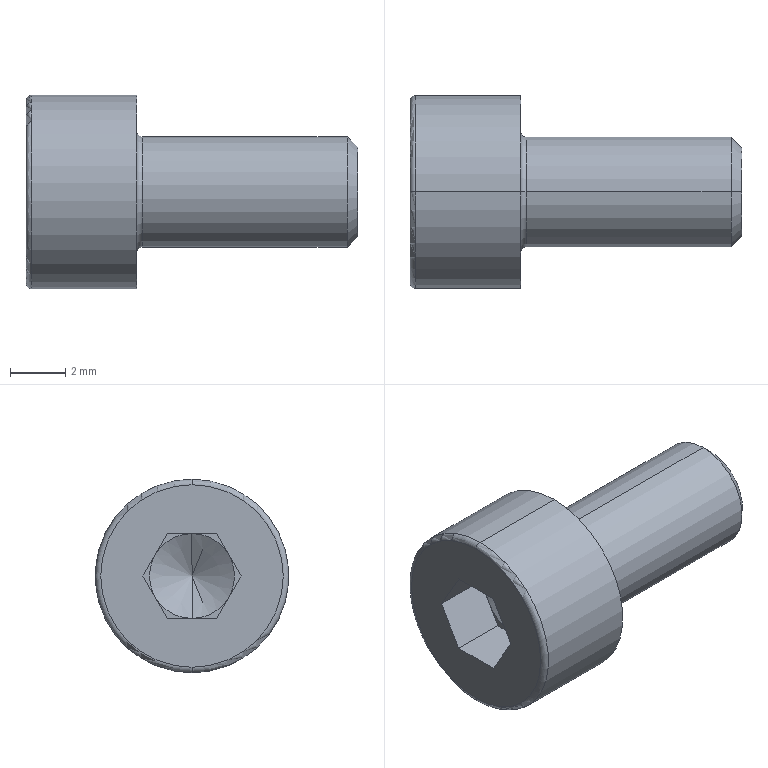Part | STEP file | socket head cap screw_iso_ISO 4762 M4 x 8 --- 8N | 1 solid | 27 faces | box 12 x 7 x 7 mm | volume 234.975 mm3 | plane 15 | cone 4 | torus 4 | cylinder 4 | commonest cylinder face diameters 4 x2 7 x2